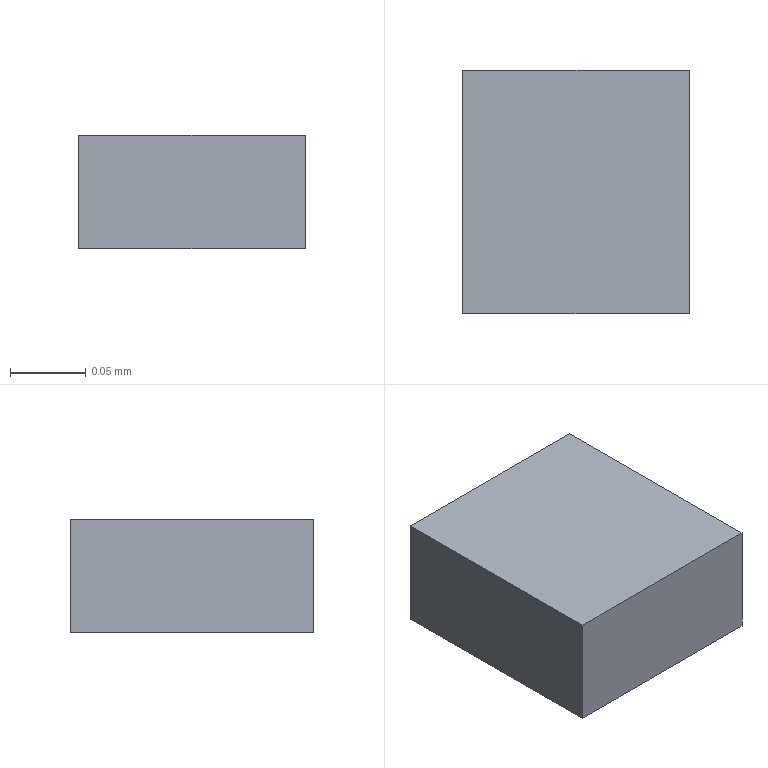Part | STEP file | RJ-USIO-V1_2-220411_347 | 1 solid | 6 faces | box 0.1489 x 0.1601 x 0.075 mm | volume 0.001787 mm3 | plane 6
STEP:
#1=CARTESIAN_POINT('',(0.,0.,0.));
#2=DIRECTION('',(0.,0.,1.));
#3=DIRECTION('',(1.,0.,0.));
#4=AXIS2_PLACEMENT_3D('',#1,#2,#3);
#5=CARTESIAN_POINT('',(60.574,66.98,0.3298));
#6=VERTEX_POINT('',#5);
#7=CARTESIAN_POINT('',(60.574,66.82,0.3298));
#8=VERTEX_POINT('',#7);
#9=CARTESIAN_POINT('',(60.574,66.98,0.3298));
#10=DIRECTION('',(0.000000175,-1.,0.));
#11=VECTOR('',#10,1.);
#12=LINE('',#9,#11);
#13=CARTESIAN_POINT('',(60.5,66.9,0.3298));
#14=DIRECTION('',(0.,0.,1.));
#15=DIRECTION('',(-1.,-0.000000175,0.));
#16=AXIS2_PLACEMENT_3D('',#13,#14,#15);
#17=PLANE('',#16);
#18=CARTESIAN_POINT('',(-0.07444,-0.08003));
#19=DIRECTION('',(0.,1.));
#20=VECTOR('',#19,1.);
#21=LINE('',#18,#20);
#22=(GEOMETRIC_REPRESENTATION_CONTEXT(2)PARAMETRIC_REPRESENTATION_CONTEXT()REPRESENTATION_CONTEXT('',''));
#23=DEFINITIONAL_REPRESENTATION('',(#21),#22);
#24=PCURVE('',#17,#23);
#25=CARTESIAN_POINT('',(60.574,66.82,0.3798));
#26=DIRECTION('',(1.,0.000000175,0.));
#27=DIRECTION('',(0.000000175,-1.,0.));
#28=AXIS2_PLACEMENT_3D('',#25,#26,#27);
#29=PLANE('',#28);
#30=CARTESIAN_POINT('',(-0.1601,0.05));
#31=DIRECTION('',(1.,0.));
#32=VECTOR('',#31,1.);
#33=LINE('',#30,#32);
#34=(GEOMETRIC_REPRESENTATION_CONTEXT(2)PARAMETRIC_REPRESENTATION_CONTEXT()REPRESENTATION_CONTEXT('',''));
#35=DEFINITIONAL_REPRESENTATION('',(#33),#34);
#36=PCURVE('',#29,#35);
#37=SURFACE_CURVE('',#12,(#24,#36),.PCURVE_S1.);
#38=EDGE_CURVE('',#6,#8,#37,.T.);
#39=ORIENTED_EDGE('',*,*,#38,.F.);
#40=CARTESIAN_POINT('',(60.425,66.98,0.3298));
#41=VERTEX_POINT('',#40);
#42=CARTESIAN_POINT('',(60.425,66.98,0.3298));
#43=DIRECTION('',(1.,0.000000175,0.));
#44=VECTOR('',#43,1.);
#45=LINE('',#42,#44);
#46=CARTESIAN_POINT('',(0.07444,-0.08003));
#47=DIRECTION('',(-1.,0.));
#48=VECTOR('',#47,1.);
#49=LINE('',#46,#48);
#50=(GEOMETRIC_REPRESENTATION_CONTEXT(2)PARAMETRIC_REPRESENTATION_CONTEXT()REPRESENTATION_CONTEXT('',''));
#51=DEFINITIONAL_REPRESENTATION('',(#49),#50);
#52=PCURVE('',#17,#51);
#53=CARTESIAN_POINT('',(60.574,66.98,0.3798));
#54=DIRECTION('',(-0.000000175,1.,0.));
#55=DIRECTION('',(1.,0.000000175,0.));
#56=AXIS2_PLACEMENT_3D('',#53,#54,#55);
#57=PLANE('',#56);
#58=CARTESIAN_POINT('',(-0.1489,0.05));
#59=DIRECTION('',(1.,0.));
#60=VECTOR('',#59,1.);
#61=LINE('',#58,#60);
#62=(GEOMETRIC_REPRESENTATION_CONTEXT(2)PARAMETRIC_REPRESENTATION_CONTEXT()REPRESENTATION_CONTEXT('',''));
#63=DEFINITIONAL_REPRESENTATION('',(#61),#62);
#64=PCURVE('',#57,#63);
#65=SURFACE_CURVE('',#45,(#52,#64),.PCURVE_S1.);
#66=EDGE_CURVE('',#41,#6,#65,.T.);
#67=ORIENTED_EDGE('',*,*,#66,.F.);
#68=CARTESIAN_POINT('',(60.425,66.82,0.3298));
#69=VERTEX_POINT('',#68);
#70=CARTESIAN_POINT('',(60.425,66.82,0.3298));
#71=DIRECTION('',(-0.000000175,1.,0.));
#72=VECTOR('',#71,1.);
#73=LINE('',#70,#72);
#74=CARTESIAN_POINT('',(0.07444,0.08003));
#75=DIRECTION('',(0.,-1.));
#76=VECTOR('',#75,1.);
#77=LINE('',#74,#76);
#78=(GEOMETRIC_REPRESENTATION_CONTEXT(2)PARAMETRIC_REPRESENTATION_CONTEXT()REPRESENTATION_CONTEXT('',''));
#79=DEFINITIONAL_REPRESENTATION('',(#77),#78);
#80=PCURVE('',#17,#79);
#81=CARTESIAN_POINT('',(60.425,66.98,0.3798));
#82=DIRECTION('',(-1.,-0.000000175,0.));
#83=DIRECTION('',(-0.000000175,1.,0.));
#84=AXIS2_PLACEMENT_3D('',#81,#82,#83);
#85=PLANE('',#84);
#86=CARTESIAN_POINT('',(-0.1601,0.05));
#87=DIRECTION('',(1.,0.));
#88=VECTOR('',#87,1.);
#89=LINE('',#86,#88);
#90=(GEOMETRIC_REPRESENTATION_CONTEXT(2)PARAMETRIC_REPRESENTATION_CONTEXT()REPRESENTATION_CONTEXT('',''));
#91=DEFINITIONAL_REPRESENTATION('',(#89),#90);
#92=PCURVE('',#85,#91);
#93=SURFACE_CURVE('',#73,(#80,#92),.PCURVE_S1.);
#94=EDGE_CURVE('',#69,#41,#93,.T.);
#95=ORIENTED_EDGE('',*,*,#94,.F.);
#96=CARTESIAN_POINT('',(60.574,66.82,0.3298));
#97=DIRECTION('',(-1.,-0.000000175,0.));
#98=VECTOR('',#97,1.);
#99=LINE('',#96,#98);
#100=CARTESIAN_POINT('',(-0.07444,0.08003));
#101=DIRECTION('',(1.,0.));
#102=VECTOR('',#101,1.);
#103=LINE('',#100,#102);
#104=(GEOMETRIC_REPRESENTATION_CONTEXT(2)PARAMETRIC_REPRESENTATION_CONTEXT()REPRESENTATION_CONTEXT('',''));
#105=DEFINITIONAL_REPRESENTATION('',(#103),#104);
#106=PCURVE('',#17,#105);
#107=CARTESIAN_POINT('',(60.574,66.82,0.3798));
#108=DIRECTION('',(0.000000175,-1.,0.));
#109=DIRECTION('',(-1.,-0.000000175,0.));
#110=AXIS2_PLACEMENT_3D('',#107,#108,#109);
#111=PLANE('',#110);
#112=CARTESIAN_POINT('',(0.,0.05));
#113=DIRECTION('',(1.,0.));
#114=VECTOR('',#113,1.);
#115=LINE('',#112,#114);
#116=(GEOMETRIC_REPRESENTATION_CONTEXT(2)PARAMETRIC_REPRESENTATION_CONTEXT()REPRESENTATION_CONTEXT('',''));
#117=DEFINITIONAL_REPRESENTATION('',(#115),#116);
#118=PCURVE('',#111,#117);
#119=SURFACE_CURVE('',#99,(#106,#118),.PCURVE_S1.);
#120=EDGE_CURVE('',#8,#69,#119,.T.);
#121=ORIENTED_EDGE('',*,*,#120,.F.);
#122=EDGE_LOOP('',(#39,#67,#95,#121));
#123=FACE_BOUND('',#122,.F.);
#124=ADVANCED_FACE('',(#123),#17,.F.);
#125=ORIENTED_EDGE('',*,*,#38,.T.);
#126=CARTESIAN_POINT('',(60.574,66.82,0.4048));
#127=VERTEX_POINT('',#126);
#128=CARTESIAN_POINT('',(60.574,66.82,0.3298));
#129=DIRECTION('',(0.,0.,1.));
#130=VECTOR('',#129,1.);
#131=LINE('',#128,#130);
#132=CARTESIAN_POINT('',(0.,0.05));
#133=DIRECTION('',(0.,-1.));
#134=VECTOR('',#133,1.);
#135=LINE('',#132,#134);
#136=(GEOMETRIC_REPRESENTATION_CONTEXT(2)PARAMETRIC_REPRESENTATION_CONTEXT()REPRESENTATION_CONTEXT('',''));
#137=DEFINITIONAL_REPRESENTATION('',(#135),#136);
#138=PCURVE('',#29,#137);
#139=CARTESIAN_POINT('',(0.,0.05));
#140=DIRECTION('',(0.,-1.));
#141=VECTOR('',#140,1.);
#142=LINE('',#139,#141);
#143=(GEOMETRIC_REPRESENTATION_CONTEXT(2)PARAMETRIC_REPRESENTATION_CONTEXT()REPRESENTATION_CONTEXT('',''));
#144=DEFINITIONAL_REPRESENTATION('',(#142),#143);
#145=PCURVE('',#111,#144);
#146=SURFACE_CURVE('',#131,(#138,#145),.PCURVE_S1.);
#147=EDGE_CURVE('',#8,#127,#146,.T.);
#148=ORIENTED_EDGE('',*,*,#147,.T.);
#149=CARTESIAN_POINT('',(60.574,66.98,0.4048));
#150=VERTEX_POINT('',#149);
#151=CARTESIAN_POINT('',(60.574,66.82,0.4048));
#152=DIRECTION('',(-0.000000175,1.,0.));
#153=VECTOR('',#152,1.);
#154=LINE('',#151,#153);
#155=CARTESIAN_POINT('',(0.,-0.025));
#156=DIRECTION('',(-1.,0.));
#157=VECTOR('',#156,1.);
#158=LINE('',#155,#157);
#159=(GEOMETRIC_REPRESENTATION_CONTEXT(2)PARAMETRIC_REPRESENTATION_CONTEXT()REPRESENTATION_CONTEXT('',''));
#160=DEFINITIONAL_REPRESENTATION('',(#158),#159);
#161=PCURVE('',#29,#160);
#162=CARTESIAN_POINT('',(60.5,66.9,0.4048));
#163=DIRECTION('',(0.,0.,1.));
#164=DIRECTION('',(-1.,-0.000000175,0.));
#165=AXIS2_PLACEMENT_3D('',#162,#163,#164);
#166=PLANE('',#165);
#167=CARTESIAN_POINT('',(-0.07444,0.08003));
#168=DIRECTION('',(0.,-1.));
#169=VECTOR('',#168,1.);
#170=LINE('',#167,#169);
#171=(GEOMETRIC_REPRESENTATION_CONTEXT(2)PARAMETRIC_REPRESENTATION_CONTEXT()REPRESENTATION_CONTEXT('',''));
#172=DEFINITIONAL_REPRESENTATION('',(#170),#171);
#173=PCURVE('',#166,#172);
#174=SURFACE_CURVE('',#154,(#161,#173),.PCURVE_S1.);
#175=EDGE_CURVE('',#127,#150,#174,.T.);
#176=ORIENTED_EDGE('',*,*,#175,.T.);
#177=CARTESIAN_POINT('',(60.574,66.98,0.3298));
#178=DIRECTION('',(0.,0.,1.));
#179=VECTOR('',#178,1.);
#180=LINE('',#177,#179);
#181=CARTESIAN_POINT('',(-0.1601,0.05));
#182=DIRECTION('',(0.,-1.));
#183=VECTOR('',#182,1.);
#184=LINE('',#181,#183);
#185=(GEOMETRIC_REPRESENTATION_CONTEXT(2)PARAMETRIC_REPRESENTATION_CONTEXT()REPRESENTATION_CONTEXT('',''));
#186=DEFINITIONAL_REPRESENTATION('',(#184),#185);
#187=PCURVE('',#29,#186);
#188=CARTESIAN_POINT('',(0.,0.05));
#189=DIRECTION('',(0.,-1.));
#190=VECTOR('',#189,1.);
#191=LINE('',#188,#190);
#192=(GEOMETRIC_REPRESENTATION_CONTEXT(2)PARAMETRIC_REPRESENTATION_CONTEXT()REPRESENTATION_CONTEXT('',''));
#193=DEFINITIONAL_REPRESENTATION('',(#191),#192);
#194=PCURVE('',#57,#193);
#195=SURFACE_CURVE('',#180,(#187,#194),.PCURVE_S1.);
#196=EDGE_CURVE('',#6,#150,#195,.T.);
#197=ORIENTED_EDGE('',*,*,#196,.F.);
#198=EDGE_LOOP('',(#125,#148,#176,#197));
#199=FACE_BOUND('',#198,.F.);
#200=ADVANCED_FACE('',(#199),#29,.T.);
#201=CARTESIAN_POINT('',(60.425,66.82,0.4048));
#202=VERTEX_POINT('',#201);
#203=CARTESIAN_POINT('',(60.425,66.82,0.4048));
#204=DIRECTION('',(1.,0.000000175,0.));
#205=VECTOR('',#204,1.);
#206=LINE('',#203,#205);
#207=CARTESIAN_POINT('',(0.1489,-0.025));
#208=DIRECTION('',(-1.,0.));
#209=VECTOR('',#208,1.);
#210=LINE('',#207,#209);
#211=(GEOMETRIC_REPRESENTATION_CONTEXT(2)PARAMETRIC_REPRESENTATION_CONTEXT()REPRESENTATION_CONTEXT('',''));
#212=DEFINITIONAL_REPRESENTATION('',(#210),#211);
#213=PCURVE('',#111,#212);
#214=CARTESIAN_POINT('',(0.07444,0.08003));
#215=DIRECTION('',(-1.,0.));
#216=VECTOR('',#215,1.);
#217=LINE('',#214,#216);
#218=(GEOMETRIC_REPRESENTATION_CONTEXT(2)PARAMETRIC_REPRESENTATION_CONTEXT()REPRESENTATION_CONTEXT('',''));
#219=DEFINITIONAL_REPRESENTATION('',(#217),#218);
#220=PCURVE('',#166,#219);
#221=SURFACE_CURVE('',#206,(#213,#220),.PCURVE_S1.);
#222=EDGE_CURVE('',#202,#127,#221,.T.);
#223=ORIENTED_EDGE('',*,*,#222,.T.);
#224=ORIENTED_EDGE('',*,*,#147,.F.);
#225=ORIENTED_EDGE('',*,*,#120,.T.);
#226=CARTESIAN_POINT('',(60.425,66.82,0.3298));
#227=DIRECTION('',(0.,0.,1.));
#228=VECTOR('',#227,1.);
#229=LINE('',#226,#228);
#230=CARTESIAN_POINT('',(0.1489,0.05));
#231=DIRECTION('',(0.,-1.));
#232=VECTOR('',#231,1.);
#233=LINE('',#230,#232);
#234=(GEOMETRIC_REPRESENTATION_CONTEXT(2)PARAMETRIC_REPRESENTATION_CONTEXT()REPRESENTATION_CONTEXT('',''));
#235=DEFINITIONAL_REPRESENTATION('',(#233),#234);
#236=PCURVE('',#111,#235);
#237=CARTESIAN_POINT('',(-0.1601,0.05));
#238=DIRECTION('',(0.,-1.));
#239=VECTOR('',#238,1.);
#240=LINE('',#237,#239);
#241=(GEOMETRIC_REPRESENTATION_CONTEXT(2)PARAMETRIC_REPRESENTATION_CONTEXT()REPRESENTATION_CONTEXT('',''));
#242=DEFINITIONAL_REPRESENTATION('',(#240),#241);
#243=PCURVE('',#85,#242);
#244=SURFACE_CURVE('',#229,(#236,#243),.PCURVE_S1.);
#245=EDGE_CURVE('',#69,#202,#244,.T.);
#246=ORIENTED_EDGE('',*,*,#245,.T.);
#247=EDGE_LOOP('',(#223,#224,#225,#246));
#248=FACE_BOUND('',#247,.F.);
#249=ADVANCED_FACE('',(#248),#111,.T.);
#250=ORIENTED_EDGE('',*,*,#175,.F.);
#251=ORIENTED_EDGE('',*,*,#222,.F.);
#252=CARTESIAN_POINT('',(60.425,66.98,0.4048));
#253=VERTEX_POINT('',#252);
#254=CARTESIAN_POINT('',(60.425,66.98,0.4048));
#255=DIRECTION('',(0.000000175,-1.,0.));
#256=VECTOR('',#255,1.);
#257=LINE('',#254,#256);
#258=CARTESIAN_POINT('',(0.07444,-0.08003));
#259=DIRECTION('',(0.,1.));
#260=VECTOR('',#259,1.);
#261=LINE('',#258,#260);
#262=(GEOMETRIC_REPRESENTATION_CONTEXT(2)PARAMETRIC_REPRESENTATION_CONTEXT()REPRESENTATION_CONTEXT('',''));
#263=DEFINITIONAL_REPRESENTATION('',(#261),#262);
#264=PCURVE('',#166,#263);
#265=CARTESIAN_POINT('',(0.,-0.025));
#266=DIRECTION('',(-1.,0.));
#267=VECTOR('',#266,1.);
#268=LINE('',#265,#267);
#269=(GEOMETRIC_REPRESENTATION_CONTEXT(2)PARAMETRIC_REPRESENTATION_CONTEXT()REPRESENTATION_CONTEXT('',''));
#270=DEFINITIONAL_REPRESENTATION('',(#268),#269);
#271=PCURVE('',#85,#270);
#272=SURFACE_CURVE('',#257,(#264,#271),.PCURVE_S1.);
#273=EDGE_CURVE('',#253,#202,#272,.T.);
#274=ORIENTED_EDGE('',*,*,#273,.F.);
#275=CARTESIAN_POINT('',(60.574,66.98,0.4048));
#276=DIRECTION('',(-1.,-0.000000175,0.));
#277=VECTOR('',#276,1.);
#278=LINE('',#275,#277);
#279=CARTESIAN_POINT('',(-0.07444,-0.08003));
#280=DIRECTION('',(1.,0.));
#281=VECTOR('',#280,1.);
#282=LINE('',#279,#281);
#283=(GEOMETRIC_REPRESENTATION_CONTEXT(2)PARAMETRIC_REPRESENTATION_CONTEXT()REPRESENTATION_CONTEXT('',''));
#284=DEFINITIONAL_REPRESENTATION('',(#282),#283);
#285=PCURVE('',#166,#284);
#286=CARTESIAN_POINT('',(0.,-0.025));
#287=DIRECTION('',(-1.,0.));
#288=VECTOR('',#287,1.);
#289=LINE('',#286,#288);
#290=(GEOMETRIC_REPRESENTATION_CONTEXT(2)PARAMETRIC_REPRESENTATION_CONTEXT()REPRESENTATION_CONTEXT('',''));
#291=DEFINITIONAL_REPRESENTATION('',(#289),#290);
#292=PCURVE('',#57,#291);
#293=SURFACE_CURVE('',#278,(#285,#292),.PCURVE_S1.);
#294=EDGE_CURVE('',#150,#253,#293,.T.);
#295=ORIENTED_EDGE('',*,*,#294,.F.);
#296=EDGE_LOOP('',(#250,#251,#274,#295));
#297=FACE_BOUND('',#296,.F.);
#298=ADVANCED_FACE('',(#297),#166,.T.);
#299=ORIENTED_EDGE('',*,*,#273,.T.);
#300=ORIENTED_EDGE('',*,*,#245,.F.);
#301=ORIENTED_EDGE('',*,*,#94,.T.);
#302=CARTESIAN_POINT('',(60.425,66.98,0.4048));
#303=DIRECTION('',(0.,0.,-1.));
#304=VECTOR('',#303,1.);
#305=LINE('',#302,#304);
#306=CARTESIAN_POINT('',(0.,-0.025));
#307=DIRECTION('',(0.,1.));
#308=VECTOR('',#307,1.);
#309=LINE('',#306,#308);
#310=(GEOMETRIC_REPRESENTATION_CONTEXT(2)PARAMETRIC_REPRESENTATION_CONTEXT()REPRESENTATION_CONTEXT('',''));
#311=DEFINITIONAL_REPRESENTATION('',(#309),#310);
#312=PCURVE('',#85,#311);
#313=CARTESIAN_POINT('',(-0.1489,-0.025));
#314=DIRECTION('',(0.,1.));
#315=VECTOR('',#314,1.);
#316=LINE('',#313,#315);
#317=(GEOMETRIC_REPRESENTATION_CONTEXT(2)PARAMETRIC_REPRESENTATION_CONTEXT()REPRESENTATION_CONTEXT('',''));
#318=DEFINITIONAL_REPRESENTATION('',(#316),#317);
#319=PCURVE('',#57,#318);
#320=SURFACE_CURVE('',#305,(#312,#319),.PCURVE_S1.);
#321=EDGE_CURVE('',#253,#41,#320,.T.);
#322=ORIENTED_EDGE('',*,*,#321,.F.);
#323=EDGE_LOOP('',(#299,#300,#301,#322));
#324=FACE_BOUND('',#323,.F.);
#325=ADVANCED_FACE('',(#324),#85,.T.);
#326=ORIENTED_EDGE('',*,*,#294,.T.);
#327=ORIENTED_EDGE('',*,*,#321,.T.);
#328=ORIENTED_EDGE('',*,*,#66,.T.);
#329=ORIENTED_EDGE('',*,*,#196,.T.);
#330=EDGE_LOOP('',(#326,#327,#328,#329));
#331=FACE_BOUND('',#330,.F.);
#332=ADVANCED_FACE('',(#331),#57,.T.);
#333=CLOSED_SHELL('',(#124,#200,#249,#298,#325,#332));
#334=MANIFOLD_SOLID_BREP('',#333);
#335=(LENGTH_UNIT()NAMED_UNIT(*)SI_UNIT(.MILLI.,.METRE.));
#336=UNCERTAINTY_MEASURE_WITH_UNIT(LENGTH_MEASURE(0.0000001),#335,'','');
#337=(NAMED_UNIT(*)PLANE_ANGLE_UNIT()SI_UNIT($,.RADIAN.));
#338=(NAMED_UNIT(*)SI_UNIT($,.STERADIAN.)SOLID_ANGLE_UNIT());
#339=(GEOMETRIC_REPRESENTATION_CONTEXT(3)GLOBAL_UNCERTAINTY_ASSIGNED_CONTEXT((#336))GLOBAL_UNIT_ASSIGNED_CONTEXT((#335,#337,#338))REPRESENTATION_CONTEXT('',''));
#340=ADVANCED_BREP_SHAPE_REPRESENTATION('',(#4,#334),#339);